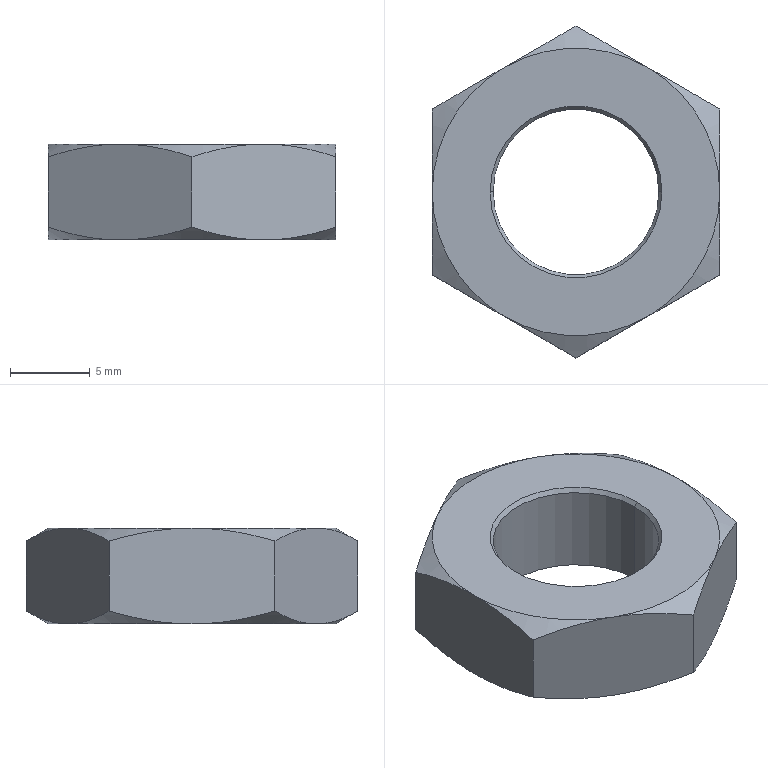Part | STEP file | 1 solid | 26 faces | box 18 x 20.785 x 6 mm | volume 1162 mm3 | cone 16 | plane 8 | cylinder 2 | commonest cylinder face diameters 10.376 x2